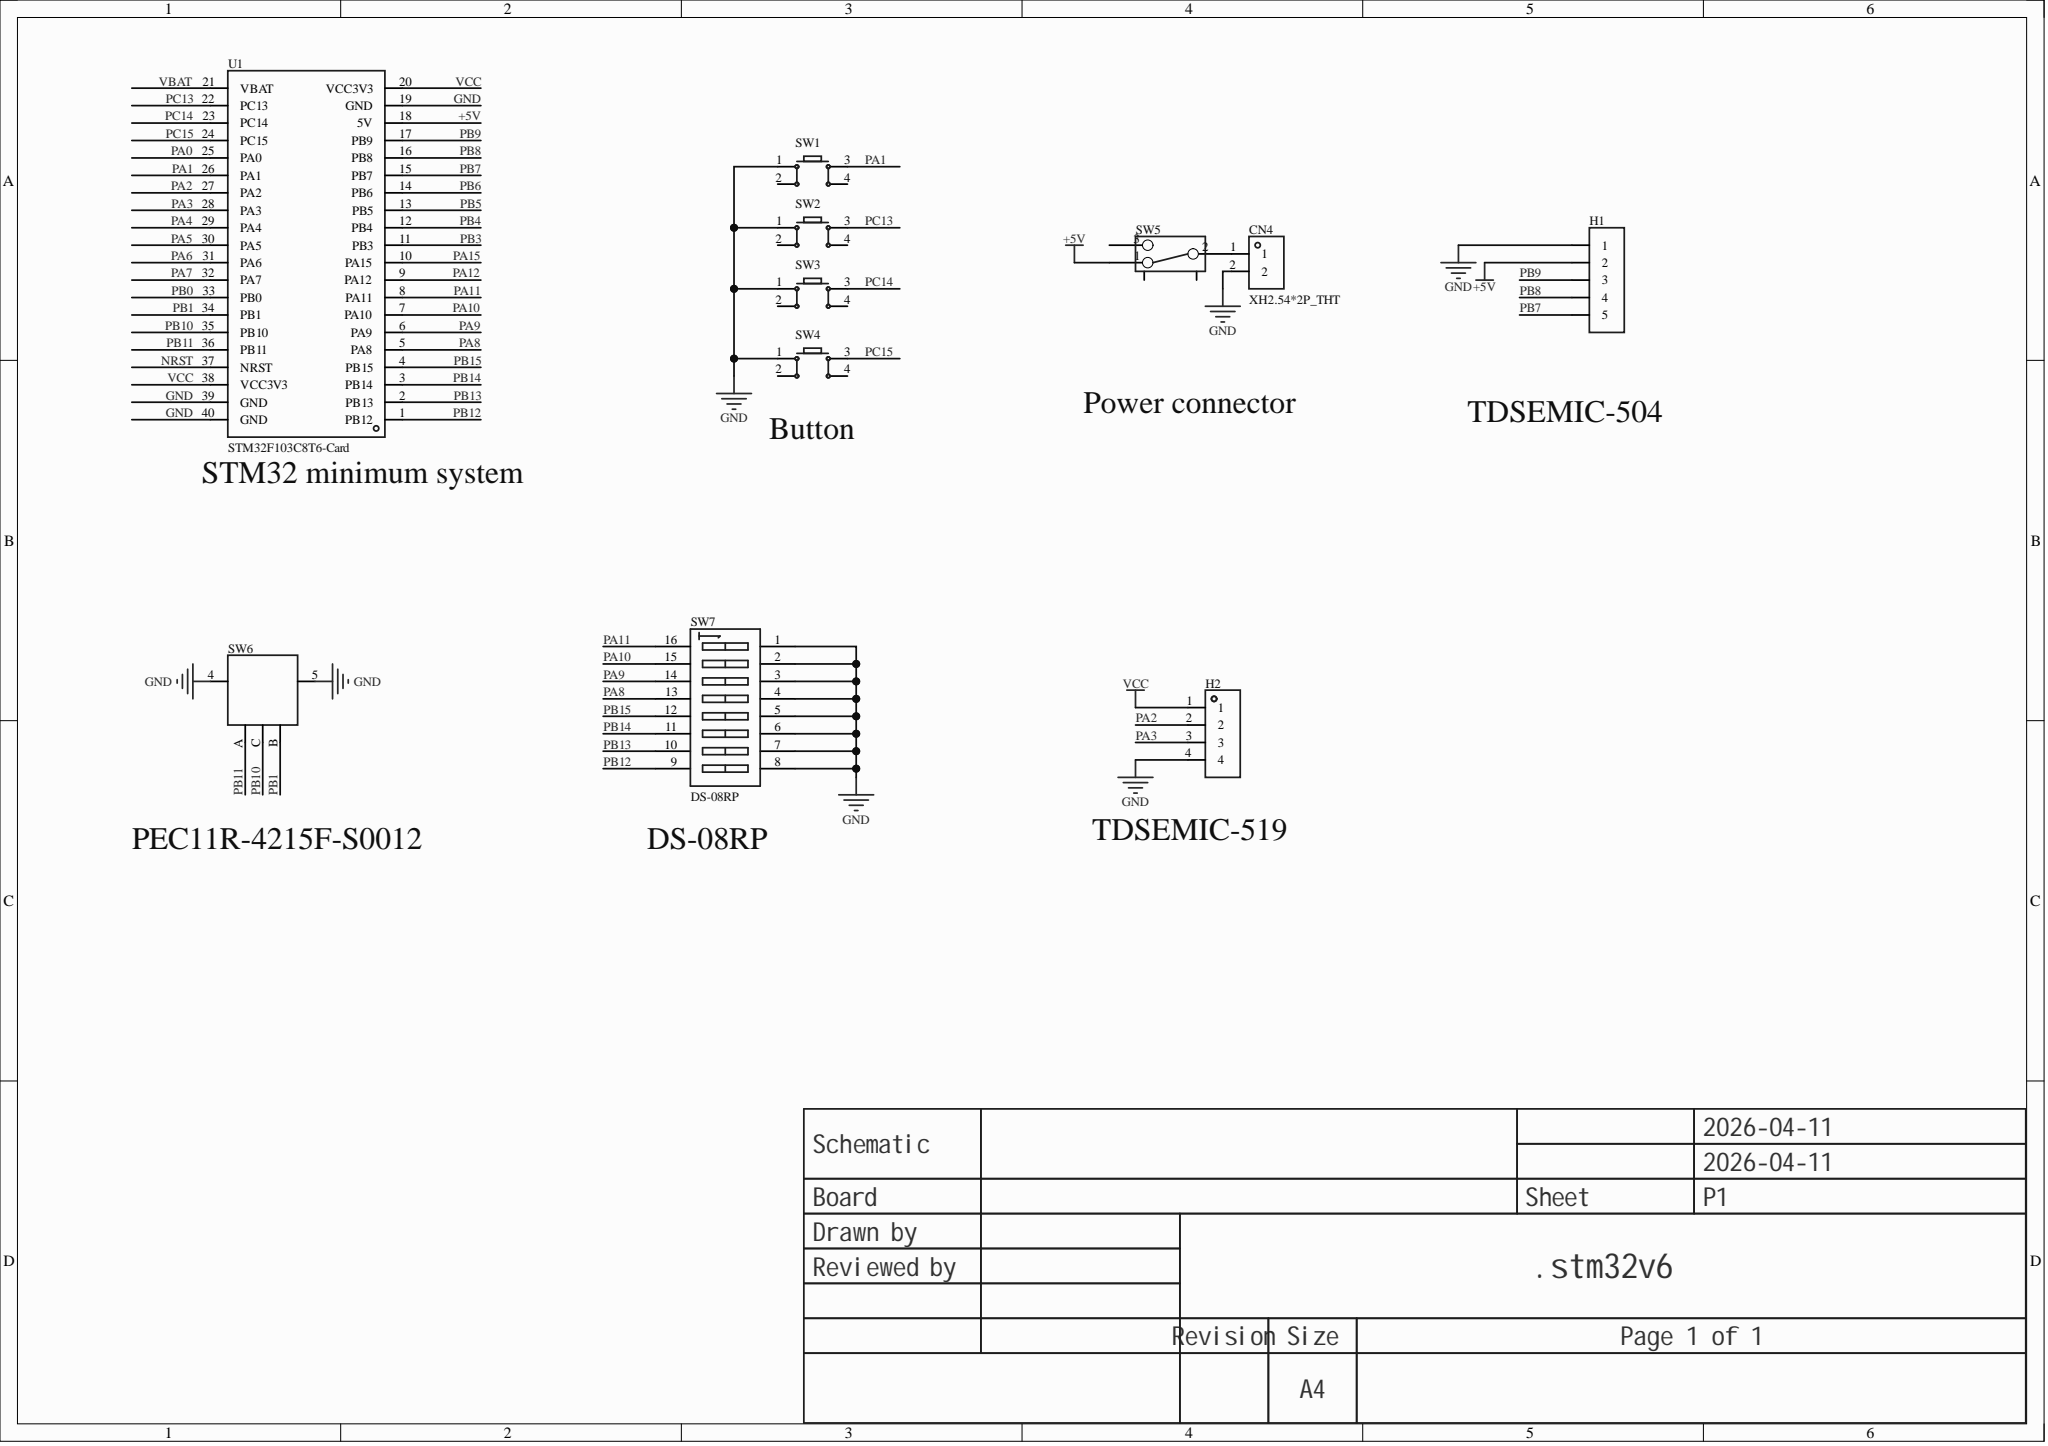Circuit board | Altium Designer | 11 parts | 24 nets
Bill of materials:
Comment,Description,Designator,Footprint,LibRef,Quantity
"XH2.54*2P_THT","","CN4","CONN-TH_2P-P2.50-XH2.54-2P","XH2.54*2P_直插","1"
"","","H1","HDR-TH_5P-P2.54-V-F","HDR-F_2.54_1x5P","1"
"","","H2","HDR-TH_4P-P2.54-V-F","HDR-F_2.54_1x4P","1"
"","","SW1, SW2, SW3, SW4","SW-TH_4P-L6.0-W6.0-P4.50-LS6.5","Key_TH_6x6x6","4"
"","","SW5","拨动开关","拨动开关_正","1"
"PEC11R-4215F-N0024","","SW6","SW-TH_PEC11R-4215F-N0024","PEC11R-4215F-N0024","1"
"DS-08RP","Type: flat toggle, raised; Circuit: SPST; Positions: 8; Rated current:25mA; Rated voltage:24V; Operating life:3 thousand cycles; Colour: red;","SW7","SW-TH_DS-08XP","DS-08RP","1"
"STM32F103C8T6-Card","","U1","CONN-TH_L53.3-W22.9_STM32F103C8T6-CARD","STM32F103C8T6-Card","1"
Netlist (Protel format):
[
CN4
CONN-TH_2P-P2.50-XH2.54-2P
XH2.54*2P_THT



]
[
H1
HDR-TH_5P-P2.54-V-F




]
[
H2
HDR-TH_4P-P2.54-V-F




]
[
SW1
SW-TH_4P-L6.0-W6.0-P4.50-LS6.5




]
[
SW2
SW-TH_4P-L6.0-W6.0-P4.50-LS6.5




]
[
SW3
SW-TH_4P-L6.0-W6.0-P4.50-LS6.5




]
[
SW4
SW-TH_4P-L6.0-W6.0-P4.50-LS6.5




]
[
SW5
拨动开关




]
[
SW6
SW-TH_PEC11R-4215F-N0024
PEC11R-4215F-N0024



]
[
SW7
SW-TH_DS-08XP
DS-08RP



]
[
U1
CONN-TH_L53.3-W22.9_STM32F103C8T6-CARD
STM32F103C8T6-Card



]
(
VCC
H2-1
U1-20
U1-38
)
(
PC15
SW4-3
U1-24
)
(
PC14
SW3-3
U1-23
)
(
PC13
SW2-3
U1-22
)
(
PB15
SW7-12
U1-4
)
(
PB14
SW7-11
U1-3
)
(
PB13
SW7-10
U1-2
)
(
PB12
SW7-9
U1-1
)
(
PB11
SW6-A
U1-36
)
(
PB10
SW6-C
U1-35
)
(
PB9
H1-3
U1-17
)
(
PB8
H1-4
U1-16
)
(
PB7
H1-5
U1-15
)
(
PB1
SW6-B
U1-34
)
(
PA11
SW7-16
U1-8
)
(
PA10
SW7-15
U1-7
)
(
PA9
SW7-14
U1-6
)
(
PA8
SW7-13
U1-5
)
(
PA3
H2-3
U1-28
)
(
PA2
H2-2
U1-27
)
(
PA1
SW1-3
U1-26
)
(
NetCN4_1
CN4-1
SW5-2
)
(
GND
CN4-2
H1-1
H2-4
SW1-1
SW2-1
SW3-1
SW4-1
SW6-4
SW6-5
SW7-1
SW7-2
SW7-3
SW7-4
SW7-5
SW7-6
SW7-7
SW7-8
U1-19
U1-39
U1-40
)
(
+5V
H1-2
SW5-1
U1-18
)